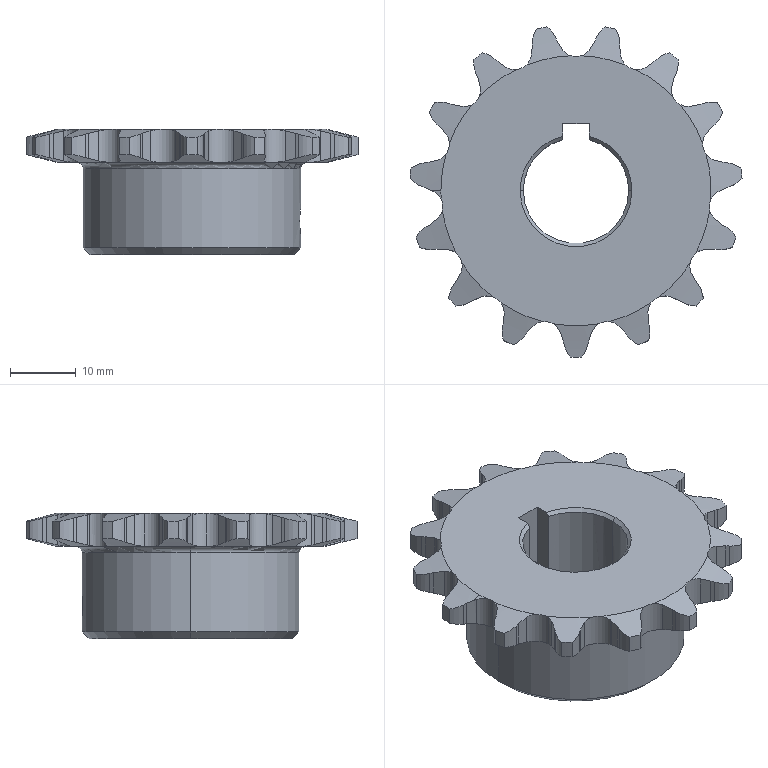Part | STEP file | BZJ-LSX-RGX 主动链轮06B-15齿_内Holeφ16 | 1 solid | 187 faces | box 50.395 x 50.132 x 19 mm | volume 15455 mm3 | cylinder 106 | cone 40 | plane 39 | torus 2 | commonest cylinder face diameters 8.515 x32 13.236 x31 5.108 x19 50.527 x15 4.2 x4 16 x3